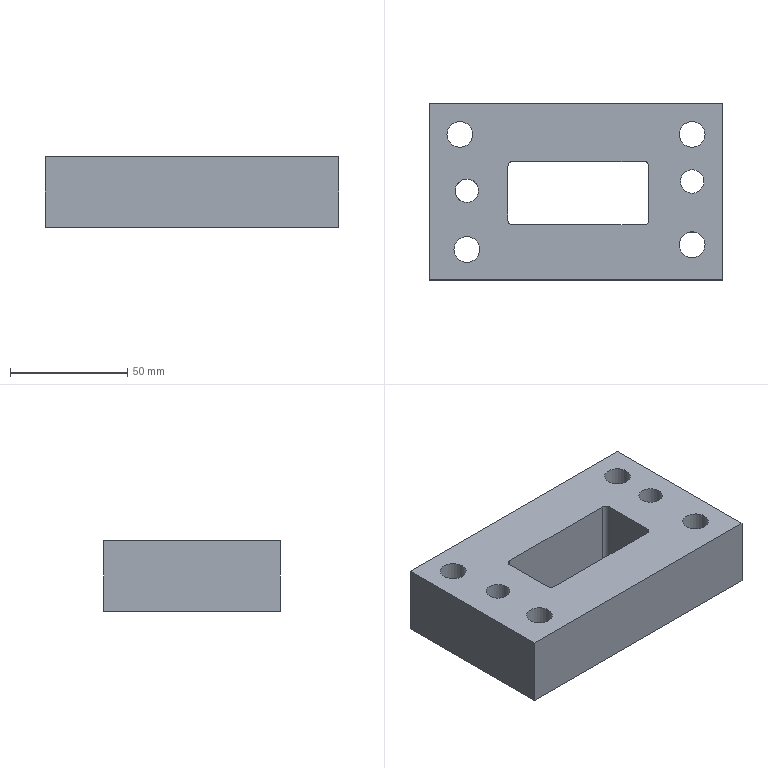Part | STEP file | 211_id690_x_t | 1 solid | 32 faces | box 125 x 75 x 30 mm | volume 208225 mm3 | plane 16 | cylinder 16 | commonest cylinder face diameters 11 x6 4 x4 17 x4 10 x2